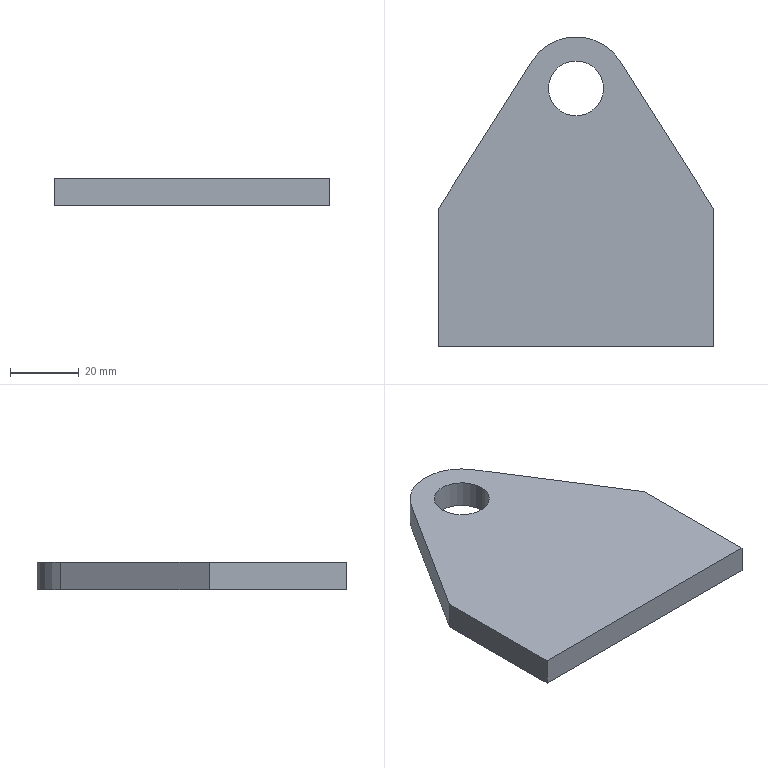Part | SolidWorks | features Extrusion 1 | 1 solid | 10 faces | box 80 x 90 x 8 mm | volume 43119 mm3 | plane 7 | cylinder 3 | commonest cylinder face diameters 16 x2 30 x1
STEP:
#1=CARTESIAN_POINT('',(32.,75.,8.));
#2=VERTEX_POINT('',#1);
#3=CARTESIAN_POINT('',(48.,75.,8.));
#4=VERTEX_POINT('',#3);
#5=CARTESIAN_POINT('',(40.,75.,8.));
#6=DIRECTION('',(0.,0.,1.));
#7=DIRECTION('',(1.,0.,0.));
#8=AXIS2_PLACEMENT_3D('',#5,#6,#7);
#9=CIRCLE('',#8,8.);
#10=EDGE_CURVE('',#2,#4,#9,.T.);
#11=ORIENTED_EDGE('',*,*,#10,.T.);
#12=CARTESIAN_POINT('',(48.,75.,0.));
#13=VERTEX_POINT('',#12);
#14=CARTESIAN_POINT('',(48.,75.,8.));
#15=DIRECTION('',(0.,0.,-1.));
#16=VECTOR('',#15,1000.);
#17=LINE('',#14,#16);
#18=EDGE_CURVE('',#4,#13,#17,.T.);
#19=ORIENTED_EDGE('',*,*,#18,.T.);
#20=CARTESIAN_POINT('',(32.,75.,0.));
#21=VERTEX_POINT('',#20);
#22=CARTESIAN_POINT('',(40.,75.,0.));
#23=DIRECTION('',(0.,0.,1.));
#24=DIRECTION('',(1.,0.,0.));
#25=AXIS2_PLACEMENT_3D('',#22,#23,#24);
#26=CIRCLE('',#25,8.);
#27=EDGE_CURVE('',#21,#13,#26,.T.);
#28=ORIENTED_EDGE('',*,*,#27,.F.);
#29=CARTESIAN_POINT('',(32.,75.,8.));
#30=DIRECTION('',(0.,0.,-1.));
#31=VECTOR('',#30,1000.);
#32=LINE('',#29,#31);
#33=EDGE_CURVE('',#2,#21,#32,.T.);
#34=ORIENTED_EDGE('',*,*,#33,.F.);
#35=EDGE_LOOP('',(#11,#19,#28,#34));
#36=FACE_OUTER_BOUND('',#35,.T.);
#37=CARTESIAN_POINT('',(40.,75.,8.));
#38=DIRECTION('',(0.,0.,-1.));
#39=DIRECTION('',(-1.,0.,0.));
#40=AXIS2_PLACEMENT_3D('',#37,#38,#39);
#41=CYLINDRICAL_SURFACE('',#40,8.);
#42=ADVANCED_FACE('',(#36),#41,.F.);
#43=CARTESIAN_POINT('',(0.,0.,8.));
#44=VERTEX_POINT('',#43);
#45=CARTESIAN_POINT('',(80.,0.,8.));
#46=VERTEX_POINT('',#45);
#47=CARTESIAN_POINT('',(0.,0.,8.));
#48=DIRECTION('',(1.,0.,0.));
#49=VECTOR('',#48,1000.);
#50=LINE('',#47,#49);
#51=EDGE_CURVE('',#44,#46,#50,.T.);
#52=ORIENTED_EDGE('',*,*,#51,.T.);
#53=CARTESIAN_POINT('',(80.,40.,8.));
#54=VERTEX_POINT('',#53);
#55=CARTESIAN_POINT('',(80.,0.,8.));
#56=DIRECTION('',(0.,1.,0.));
#57=VECTOR('',#56,1000.);
#58=LINE('',#55,#57);
#59=EDGE_CURVE('',#46,#54,#58,.T.);
#60=ORIENTED_EDGE('',*,*,#59,.T.);
#61=CARTESIAN_POINT('',(52.662,83.042,8.));
#62=VERTEX_POINT('',#61);
#63=CARTESIAN_POINT('',(80.,40.,8.));
#64=DIRECTION('',(-0.5361,0.8441,0.));
#65=VECTOR('',#64,1000.);
#66=LINE('',#63,#65);
#67=EDGE_CURVE('',#54,#62,#66,.T.);
#68=ORIENTED_EDGE('',*,*,#67,.T.);
#69=CARTESIAN_POINT('',(27.338,83.042,8.));
#70=VERTEX_POINT('',#69);
#71=CARTESIAN_POINT('',(40.,75.,8.));
#72=DIRECTION('',(0.,0.,1.));
#73=DIRECTION('',(1.,0.,0.));
#74=AXIS2_PLACEMENT_3D('',#71,#72,#73);
#75=CIRCLE('',#74,15.);
#76=EDGE_CURVE('',#62,#70,#75,.T.);
#77=ORIENTED_EDGE('',*,*,#76,.T.);
#78=CARTESIAN_POINT('',(0.,40.,8.));
#79=VERTEX_POINT('',#78);
#80=CARTESIAN_POINT('',(0.,40.,8.));
#81=DIRECTION('',(-0.5361,-0.8441,0.));
#82=VECTOR('',#81,1000.);
#83=LINE('',#80,#82);
#84=EDGE_CURVE('',#70,#79,#83,.T.);
#85=ORIENTED_EDGE('',*,*,#84,.T.);
#86=CARTESIAN_POINT('',(0.,0.,8.));
#87=DIRECTION('',(0.,-1.,0.));
#88=VECTOR('',#87,1000.);
#89=LINE('',#86,#88);
#90=EDGE_CURVE('',#79,#44,#89,.T.);
#91=ORIENTED_EDGE('',*,*,#90,.T.);
#92=EDGE_LOOP('',(#52,#60,#68,#77,#85,#91));
#93=FACE_OUTER_BOUND('',#92,.T.);
#94=ORIENTED_EDGE('',*,*,#10,.F.);
#95=CARTESIAN_POINT('',(40.,75.,8.));
#96=DIRECTION('',(0.,0.,1.));
#97=DIRECTION('',(1.,0.,0.));
#98=AXIS2_PLACEMENT_3D('',#95,#96,#97);
#99=CIRCLE('',#98,8.);
#100=EDGE_CURVE('',#4,#2,#99,.T.);
#101=ORIENTED_EDGE('',*,*,#100,.F.);
#102=EDGE_LOOP('',(#94,#101));
#103=FACE_BOUND('',#102,.T.);
#104=CARTESIAN_POINT('',(40.,75.,8.));
#105=DIRECTION('',(0.,0.,1.));
#106=DIRECTION('',(1.,0.,0.));
#107=AXIS2_PLACEMENT_3D('',#104,#105,#106);
#108=PLANE('',#107);
#109=ADVANCED_FACE('',(#93,#103),#108,.T.);
#110=CARTESIAN_POINT('',(0.,0.,0.));
#111=VERTEX_POINT('',#110);
#112=CARTESIAN_POINT('',(80.,0.,0.));
#113=VERTEX_POINT('',#112);
#114=CARTESIAN_POINT('',(0.,0.,0.));
#115=DIRECTION('',(1.,0.,0.));
#116=VECTOR('',#115,1000.);
#117=LINE('',#114,#116);
#118=EDGE_CURVE('',#111,#113,#117,.T.);
#119=ORIENTED_EDGE('',*,*,#118,.F.);
#120=CARTESIAN_POINT('',(0.,40.,0.));
#121=VERTEX_POINT('',#120);
#122=CARTESIAN_POINT('',(0.,0.,0.));
#123=DIRECTION('',(0.,-1.,0.));
#124=VECTOR('',#123,1000.);
#125=LINE('',#122,#124);
#126=EDGE_CURVE('',#121,#111,#125,.T.);
#127=ORIENTED_EDGE('',*,*,#126,.F.);
#128=CARTESIAN_POINT('',(27.338,83.042,0.));
#129=VERTEX_POINT('',#128);
#130=CARTESIAN_POINT('',(0.,40.,0.));
#131=DIRECTION('',(-0.5361,-0.8441,0.));
#132=VECTOR('',#131,1000.);
#133=LINE('',#130,#132);
#134=EDGE_CURVE('',#129,#121,#133,.T.);
#135=ORIENTED_EDGE('',*,*,#134,.F.);
#136=CARTESIAN_POINT('',(52.662,83.042,0.));
#137=VERTEX_POINT('',#136);
#138=CARTESIAN_POINT('',(40.,75.,0.));
#139=DIRECTION('',(0.,0.,1.));
#140=DIRECTION('',(1.,0.,0.));
#141=AXIS2_PLACEMENT_3D('',#138,#139,#140);
#142=CIRCLE('',#141,15.);
#143=EDGE_CURVE('',#137,#129,#142,.T.);
#144=ORIENTED_EDGE('',*,*,#143,.F.);
#145=CARTESIAN_POINT('',(80.,40.,0.));
#146=VERTEX_POINT('',#145);
#147=CARTESIAN_POINT('',(80.,40.,0.));
#148=DIRECTION('',(-0.5361,0.8441,0.));
#149=VECTOR('',#148,1000.);
#150=LINE('',#147,#149);
#151=EDGE_CURVE('',#146,#137,#150,.T.);
#152=ORIENTED_EDGE('',*,*,#151,.F.);
#153=CARTESIAN_POINT('',(80.,0.,0.));
#154=DIRECTION('',(0.,1.,0.));
#155=VECTOR('',#154,1000.);
#156=LINE('',#153,#155);
#157=EDGE_CURVE('',#113,#146,#156,.T.);
#158=ORIENTED_EDGE('',*,*,#157,.F.);
#159=EDGE_LOOP('',(#119,#127,#135,#144,#152,#158));
#160=FACE_OUTER_BOUND('',#159,.T.);
#161=ORIENTED_EDGE('',*,*,#27,.T.);
#162=CARTESIAN_POINT('',(40.,75.,0.));
#163=DIRECTION('',(0.,0.,1.));
#164=DIRECTION('',(1.,0.,0.));
#165=AXIS2_PLACEMENT_3D('',#162,#163,#164);
#166=CIRCLE('',#165,8.);
#167=EDGE_CURVE('',#13,#21,#166,.T.);
#168=ORIENTED_EDGE('',*,*,#167,.T.);
#169=EDGE_LOOP('',(#161,#168));
#170=FACE_BOUND('',#169,.T.);
#171=CARTESIAN_POINT('',(40.,75.,0.));
#172=DIRECTION('',(0.,0.,1.));
#173=DIRECTION('',(1.,0.,0.));
#174=AXIS2_PLACEMENT_3D('',#171,#172,#173);
#175=PLANE('',#174);
#176=ADVANCED_FACE('',(#160,#170),#175,.F.);
#177=ORIENTED_EDGE('',*,*,#118,.T.);
#178=CARTESIAN_POINT('',(80.,0.,8.));
#179=DIRECTION('',(0.,0.,-1.));
#180=VECTOR('',#179,1000.);
#181=LINE('',#178,#180);
#182=EDGE_CURVE('',#46,#113,#181,.T.);
#183=ORIENTED_EDGE('',*,*,#182,.F.);
#184=ORIENTED_EDGE('',*,*,#51,.F.);
#185=CARTESIAN_POINT('',(0.,0.,8.));
#186=DIRECTION('',(0.,0.,-1.));
#187=VECTOR('',#186,1000.);
#188=LINE('',#185,#187);
#189=EDGE_CURVE('',#44,#111,#188,.T.);
#190=ORIENTED_EDGE('',*,*,#189,.T.);
#191=EDGE_LOOP('',(#177,#183,#184,#190));
#192=FACE_OUTER_BOUND('',#191,.T.);
#193=CARTESIAN_POINT('',(0.,0.,8.));
#194=DIRECTION('',(0.,1.,0.));
#195=DIRECTION('',(0.,0.,1.));
#196=AXIS2_PLACEMENT_3D('',#193,#194,#195);
#197=PLANE('',#196);
#198=ADVANCED_FACE('',(#192),#197,.F.);
#199=ORIENTED_EDGE('',*,*,#157,.T.);
#200=CARTESIAN_POINT('',(80.,40.,8.));
#201=DIRECTION('',(0.,0.,-1.));
#202=VECTOR('',#201,1000.);
#203=LINE('',#200,#202);
#204=EDGE_CURVE('',#54,#146,#203,.T.);
#205=ORIENTED_EDGE('',*,*,#204,.F.);
#206=ORIENTED_EDGE('',*,*,#59,.F.);
#207=ORIENTED_EDGE('',*,*,#182,.T.);
#208=EDGE_LOOP('',(#199,#205,#206,#207));
#209=FACE_OUTER_BOUND('',#208,.T.);
#210=CARTESIAN_POINT('',(80.,0.,8.));
#211=DIRECTION('',(-1.,0.,0.));
#212=DIRECTION('',(0.,0.,1.));
#213=AXIS2_PLACEMENT_3D('',#210,#211,#212);
#214=PLANE('',#213);
#215=ADVANCED_FACE('',(#209),#214,.F.);
#216=ORIENTED_EDGE('',*,*,#151,.T.);
#217=CARTESIAN_POINT('',(52.662,83.042,8.));
#218=DIRECTION('',(0.,0.,-1.));
#219=VECTOR('',#218,1000.);
#220=LINE('',#217,#219);
#221=EDGE_CURVE('',#62,#137,#220,.T.);
#222=ORIENTED_EDGE('',*,*,#221,.F.);
#223=ORIENTED_EDGE('',*,*,#67,.F.);
#224=ORIENTED_EDGE('',*,*,#204,.T.);
#225=EDGE_LOOP('',(#216,#222,#223,#224));
#226=FACE_OUTER_BOUND('',#225,.T.);
#227=CARTESIAN_POINT('',(80.,40.,8.));
#228=DIRECTION('',(-0.8441,-0.5361,0.));
#229=DIRECTION('',(0.5361,-0.8441,0.));
#230=AXIS2_PLACEMENT_3D('',#227,#228,#229);
#231=PLANE('',#230);
#232=ADVANCED_FACE('',(#226),#231,.F.);
#233=ORIENTED_EDGE('',*,*,#143,.T.);
#234=CARTESIAN_POINT('',(27.338,83.042,8.));
#235=DIRECTION('',(0.,0.,-1.));
#236=VECTOR('',#235,1000.);
#237=LINE('',#234,#236);
#238=EDGE_CURVE('',#70,#129,#237,.T.);
#239=ORIENTED_EDGE('',*,*,#238,.F.);
#240=ORIENTED_EDGE('',*,*,#76,.F.);
#241=ORIENTED_EDGE('',*,*,#221,.T.);
#242=EDGE_LOOP('',(#233,#239,#240,#241));
#243=FACE_OUTER_BOUND('',#242,.T.);
#244=CARTESIAN_POINT('',(40.,75.,8.));
#245=DIRECTION('',(0.,0.,-1.));
#246=DIRECTION('',(-1.,0.,0.));
#247=AXIS2_PLACEMENT_3D('',#244,#245,#246);
#248=CYLINDRICAL_SURFACE('',#247,15.);
#249=ADVANCED_FACE('',(#243),#248,.T.);
#250=ORIENTED_EDGE('',*,*,#134,.T.);
#251=CARTESIAN_POINT('',(0.,40.,8.));
#252=DIRECTION('',(0.,0.,-1.));
#253=VECTOR('',#252,1000.);
#254=LINE('',#251,#253);
#255=EDGE_CURVE('',#79,#121,#254,.T.);
#256=ORIENTED_EDGE('',*,*,#255,.F.);
#257=ORIENTED_EDGE('',*,*,#84,.F.);
#258=ORIENTED_EDGE('',*,*,#238,.T.);
#259=EDGE_LOOP('',(#250,#256,#257,#258));
#260=FACE_OUTER_BOUND('',#259,.T.);
#261=CARTESIAN_POINT('',(0.,40.,8.));
#262=DIRECTION('',(0.8441,-0.5361,0.));
#263=DIRECTION('',(0.5361,0.8441,0.));
#264=AXIS2_PLACEMENT_3D('',#261,#262,#263);
#265=PLANE('',#264);
#266=ADVANCED_FACE('',(#260),#265,.F.);
#267=ORIENTED_EDGE('',*,*,#126,.T.);
#268=ORIENTED_EDGE('',*,*,#189,.F.);
#269=ORIENTED_EDGE('',*,*,#90,.F.);
#270=ORIENTED_EDGE('',*,*,#255,.T.);
#271=EDGE_LOOP('',(#267,#268,#269,#270));
#272=FACE_OUTER_BOUND('',#271,.T.);
#273=CARTESIAN_POINT('',(0.,0.,8.));
#274=DIRECTION('',(1.,0.,0.));
#275=DIRECTION('',(0.,0.,-1.));
#276=AXIS2_PLACEMENT_3D('',#273,#274,#275);
#277=PLANE('',#276);
#278=ADVANCED_FACE('',(#272),#277,.F.);
#279=ORIENTED_EDGE('',*,*,#18,.F.);
#280=ORIENTED_EDGE('',*,*,#100,.T.);
#281=ORIENTED_EDGE('',*,*,#33,.T.);
#282=ORIENTED_EDGE('',*,*,#167,.F.);
#283=EDGE_LOOP('',(#279,#280,#281,#282));
#284=FACE_OUTER_BOUND('',#283,.T.);
#285=CARTESIAN_POINT('',(40.,75.,8.));
#286=DIRECTION('',(0.,0.,-1.));
#287=DIRECTION('',(-1.,0.,0.));
#288=AXIS2_PLACEMENT_3D('',#285,#286,#287);
#289=CYLINDRICAL_SURFACE('',#288,8.);
#290=ADVANCED_FACE('',(#284),#289,.F.);
#291=CLOSED_SHELL('',(#42,#109,#176,#198,#215,#232,#249,#266,#278,#290));
#292=MANIFOLD_SOLID_BREP('',#291);
#293=CARTESIAN_POINT('',(0.,0.,0.));
#294=DIRECTION('',(0.,0.,1.));
#295=DIRECTION('',(1.,0.,0.));
#296=AXIS2_PLACEMENT_3D('',#293,#294,#295);
#297=(LENGTH_UNIT()NAMED_UNIT(*)SI_UNIT(.MILLI.,.METRE.));
#298=UNCERTAINTY_MEASURE_WITH_UNIT(LENGTH_MEASURE(0.00001),#297,'','');
#299=(NAMED_UNIT(*)PLANE_ANGLE_UNIT()SI_UNIT($,.RADIAN.));
#300=(NAMED_UNIT(*)SI_UNIT($,.STERADIAN.)SOLID_ANGLE_UNIT());
#301=(GEOMETRIC_REPRESENTATION_CONTEXT(3)GLOBAL_UNCERTAINTY_ASSIGNED_CONTEXT((#298))GLOBAL_UNIT_ASSIGNED_CONTEXT((#297,#299,#300))REPRESENTATION_CONTEXT('',''));
#302=ADVANCED_BREP_SHAPE_REPRESENTATION('',(#292,#296),#301);